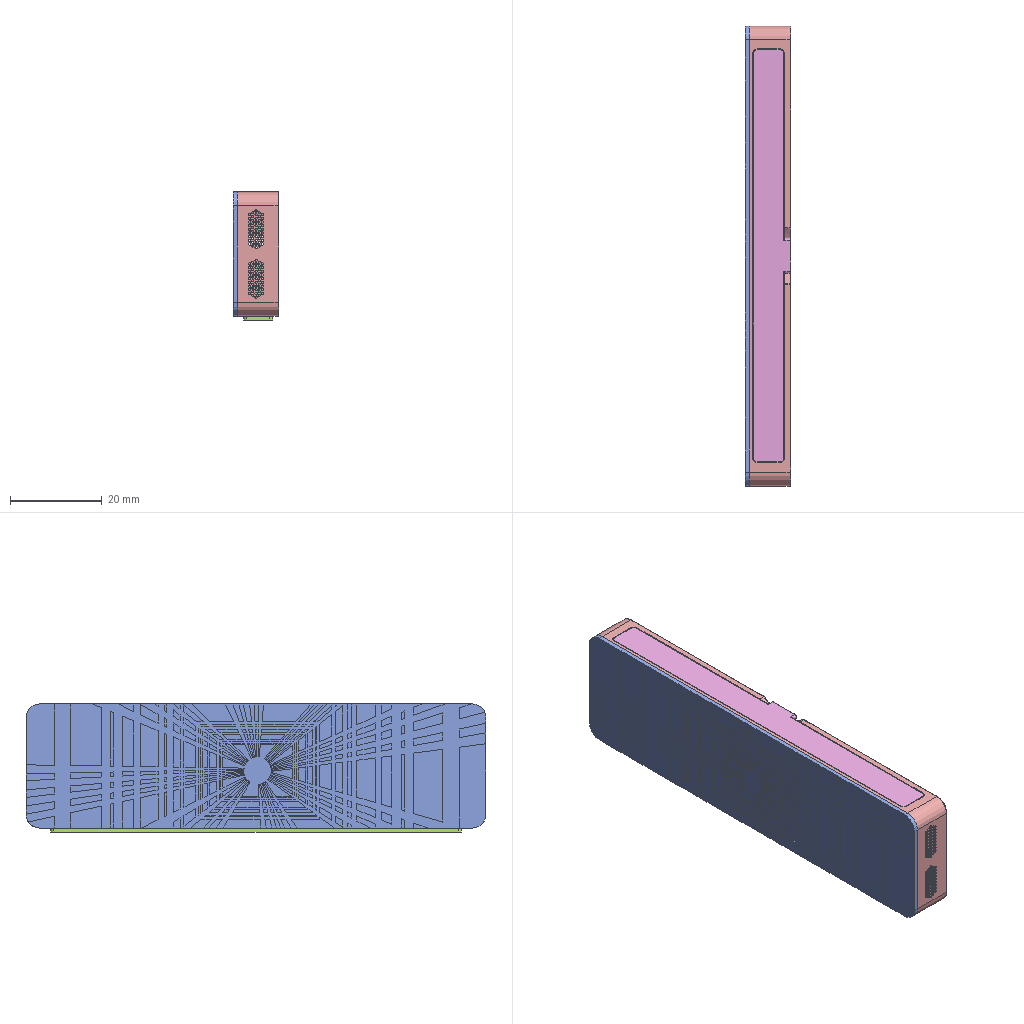Assembly | SolidWorks | 5 different items | 6 placed | box 10 x 100 x 28 mm
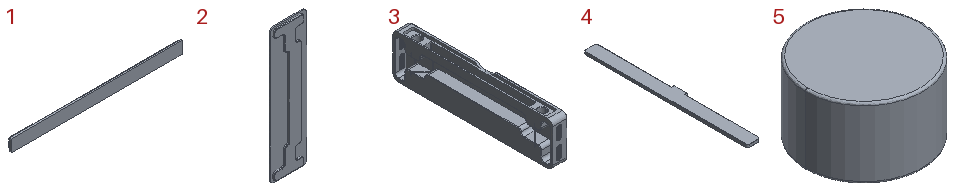Parts list (item | quantity | size | volume | features):
1 | x1 | 89.3 x 1.85 x 6.3 mm | 917.679 mm3 | features BaseBody 1
2 | x1 | 27 x 2.11 x 100 mm | 3661 mm3 | features MoveFace 2, BaseBody 1
3 | x1 | 9.09 x 100 x 27 mm | 14377 mm3 | features ICE 3, MoveFace 3, BaseBody 1, MirrorPattern 1
4 | x1 | 8.2 x 89.8 x 1.6 mm | 989.322 mm3 | features BaseBody 1, Fillet 1
5 | x2 | 5 x 5 x 3 mm | 58.841 mm3 | features BaseBody 1
Mates (type | each side: item.copy, entity, surface, feature):
Coincident | 3.1 face plane Input1 | 2.1 face plane Input1 | 3 times
Coincident | 3.1 face plane Input1 | 4.1 face plane Input1
DistanceDim | 4.1 face plane Input1 | 3.1 face plane Input1 | 2 times
Coincident | 3.1 face plane Input1 | 1.1 face plane Input1
DistanceDim | 1.1 face plane Input1 | 3.1 face plane Input1 | 2 times